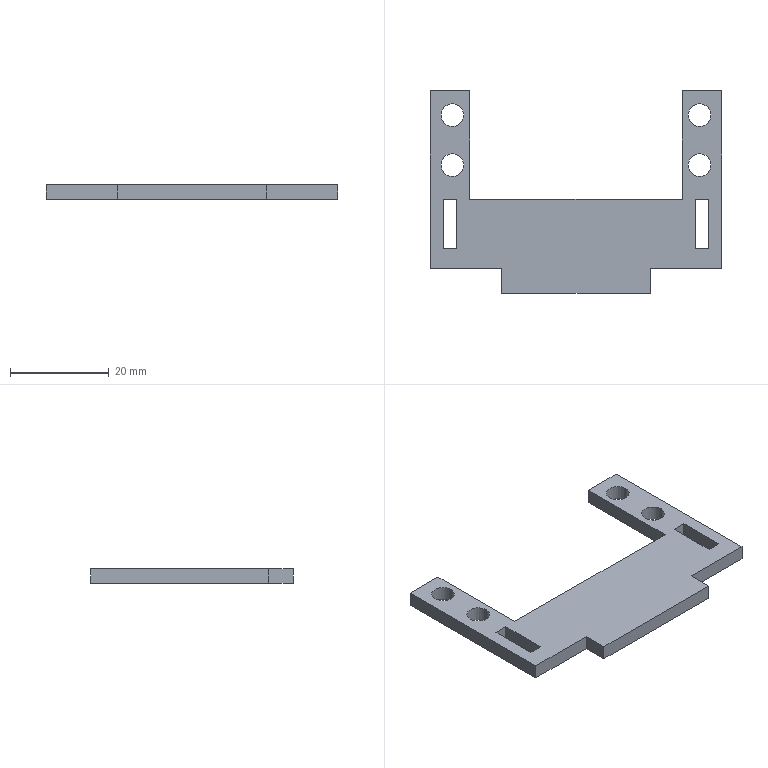Part | SolidWorks | features ICE 2, Extrusion 1 | 1 solid | 30 faces | box 59 x 41 x 3 mm | volume 3617 mm3 | plane 22 | cylinder 8 | commonest cylinder face diameters 4.6 x8
STEP:
#1=CARTESIAN_POINT('',(52.2,-15.05,3.));
#2=VERTEX_POINT('',#1);
#3=CARTESIAN_POINT('',(56.8,-15.05,3.));
#4=VERTEX_POINT('',#3);
#5=CARTESIAN_POINT('',(54.5,-15.05,3.));
#6=DIRECTION('',(0.,0.,1.));
#7=DIRECTION('',(1.,0.,0.));
#8=AXIS2_PLACEMENT_3D('',#5,#6,#7);
#9=CIRCLE('',#8,2.3);
#10=EDGE_CURVE('',#2,#4,#9,.T.);
#11=ORIENTED_EDGE('',*,*,#10,.T.);
#12=CARTESIAN_POINT('',(56.8,-15.05,0.));
#13=VERTEX_POINT('',#12);
#14=CARTESIAN_POINT('',(56.8,-15.05,3.));
#15=DIRECTION('',(0.,0.,-1.));
#16=VECTOR('',#15,1000.);
#17=LINE('',#14,#16);
#18=EDGE_CURVE('',#4,#13,#17,.T.);
#19=ORIENTED_EDGE('',*,*,#18,.T.);
#20=CARTESIAN_POINT('',(52.2,-15.05,0.));
#21=VERTEX_POINT('',#20);
#22=CARTESIAN_POINT('',(54.5,-15.05,0.));
#23=DIRECTION('',(0.,0.,1.));
#24=DIRECTION('',(1.,0.,0.));
#25=AXIS2_PLACEMENT_3D('',#22,#23,#24);
#26=CIRCLE('',#25,2.3);
#27=EDGE_CURVE('',#21,#13,#26,.T.);
#28=ORIENTED_EDGE('',*,*,#27,.F.);
#29=CARTESIAN_POINT('',(52.2,-15.05,3.));
#30=DIRECTION('',(0.,0.,-1.));
#31=VECTOR('',#30,1000.);
#32=LINE('',#29,#31);
#33=EDGE_CURVE('',#2,#21,#32,.T.);
#34=ORIENTED_EDGE('',*,*,#33,.F.);
#35=EDGE_LOOP('',(#11,#19,#28,#34));
#36=FACE_OUTER_BOUND('',#35,.T.);
#37=CARTESIAN_POINT('',(54.5,-15.05,3.));
#38=DIRECTION('',(0.,0.,-1.));
#39=DIRECTION('',(-1.,0.,0.));
#40=AXIS2_PLACEMENT_3D('',#37,#38,#39);
#41=CYLINDRICAL_SURFACE('',#40,2.3);
#42=ADVANCED_FACE('',(#36),#41,.F.);
#43=CARTESIAN_POINT('',(52.2,-4.95,3.));
#44=VERTEX_POINT('',#43);
#45=CARTESIAN_POINT('',(56.8,-4.95,3.));
#46=VERTEX_POINT('',#45);
#47=CARTESIAN_POINT('',(54.5,-4.95,3.));
#48=DIRECTION('',(0.,0.,1.));
#49=DIRECTION('',(1.,0.,0.));
#50=AXIS2_PLACEMENT_3D('',#47,#48,#49);
#51=CIRCLE('',#50,2.3);
#52=EDGE_CURVE('',#44,#46,#51,.T.);
#53=ORIENTED_EDGE('',*,*,#52,.T.);
#54=CARTESIAN_POINT('',(56.8,-4.95,0.));
#55=VERTEX_POINT('',#54);
#56=CARTESIAN_POINT('',(56.8,-4.95,3.));
#57=DIRECTION('',(0.,0.,-1.));
#58=VECTOR('',#57,1000.);
#59=LINE('',#56,#58);
#60=EDGE_CURVE('',#46,#55,#59,.T.);
#61=ORIENTED_EDGE('',*,*,#60,.T.);
#62=CARTESIAN_POINT('',(52.2,-4.95,0.));
#63=VERTEX_POINT('',#62);
#64=CARTESIAN_POINT('',(54.5,-4.95,0.));
#65=DIRECTION('',(0.,0.,1.));
#66=DIRECTION('',(1.,0.,0.));
#67=AXIS2_PLACEMENT_3D('',#64,#65,#66);
#68=CIRCLE('',#67,2.3);
#69=EDGE_CURVE('',#63,#55,#68,.T.);
#70=ORIENTED_EDGE('',*,*,#69,.F.);
#71=CARTESIAN_POINT('',(52.2,-4.95,3.));
#72=DIRECTION('',(0.,0.,-1.));
#73=VECTOR('',#72,1000.);
#74=LINE('',#71,#73);
#75=EDGE_CURVE('',#44,#63,#74,.T.);
#76=ORIENTED_EDGE('',*,*,#75,.F.);
#77=EDGE_LOOP('',(#53,#61,#70,#76));
#78=FACE_OUTER_BOUND('',#77,.T.);
#79=CARTESIAN_POINT('',(54.5,-4.95,3.));
#80=DIRECTION('',(0.,0.,-1.));
#81=DIRECTION('',(-1.,0.,0.));
#82=AXIS2_PLACEMENT_3D('',#79,#80,#81);
#83=CYLINDRICAL_SURFACE('',#82,2.3);
#84=ADVANCED_FACE('',(#78),#83,.F.);
#85=CARTESIAN_POINT('',(2.2,-4.95,3.));
#86=VERTEX_POINT('',#85);
#87=CARTESIAN_POINT('',(6.8,-4.95,3.));
#88=VERTEX_POINT('',#87);
#89=CARTESIAN_POINT('',(4.5,-4.95,3.));
#90=DIRECTION('',(0.,0.,1.));
#91=DIRECTION('',(1.,0.,0.));
#92=AXIS2_PLACEMENT_3D('',#89,#90,#91);
#93=CIRCLE('',#92,2.3);
#94=EDGE_CURVE('',#86,#88,#93,.T.);
#95=ORIENTED_EDGE('',*,*,#94,.T.);
#96=CARTESIAN_POINT('',(6.8,-4.95,0.));
#97=VERTEX_POINT('',#96);
#98=CARTESIAN_POINT('',(6.8,-4.95,3.));
#99=DIRECTION('',(0.,0.,-1.));
#100=VECTOR('',#99,1000.);
#101=LINE('',#98,#100);
#102=EDGE_CURVE('',#88,#97,#101,.T.);
#103=ORIENTED_EDGE('',*,*,#102,.T.);
#104=CARTESIAN_POINT('',(2.2,-4.95,0.));
#105=VERTEX_POINT('',#104);
#106=CARTESIAN_POINT('',(4.5,-4.95,0.));
#107=DIRECTION('',(0.,0.,1.));
#108=DIRECTION('',(1.,0.,0.));
#109=AXIS2_PLACEMENT_3D('',#106,#107,#108);
#110=CIRCLE('',#109,2.3);
#111=EDGE_CURVE('',#105,#97,#110,.T.);
#112=ORIENTED_EDGE('',*,*,#111,.F.);
#113=CARTESIAN_POINT('',(2.2,-4.95,3.));
#114=DIRECTION('',(0.,0.,-1.));
#115=VECTOR('',#114,1000.);
#116=LINE('',#113,#115);
#117=EDGE_CURVE('',#86,#105,#116,.T.);
#118=ORIENTED_EDGE('',*,*,#117,.F.);
#119=EDGE_LOOP('',(#95,#103,#112,#118));
#120=FACE_OUTER_BOUND('',#119,.T.);
#121=CARTESIAN_POINT('',(4.5,-4.95,3.));
#122=DIRECTION('',(0.,0.,-1.));
#123=DIRECTION('',(-1.,0.,0.));
#124=AXIS2_PLACEMENT_3D('',#121,#122,#123);
#125=CYLINDRICAL_SURFACE('',#124,2.3);
#126=ADVANCED_FACE('',(#120),#125,.F.);
#127=CARTESIAN_POINT('',(2.2,-15.05,3.));
#128=VERTEX_POINT('',#127);
#129=CARTESIAN_POINT('',(6.8,-15.05,3.));
#130=VERTEX_POINT('',#129);
#131=CARTESIAN_POINT('',(4.5,-15.05,3.));
#132=DIRECTION('',(0.,0.,1.));
#133=DIRECTION('',(1.,0.,0.));
#134=AXIS2_PLACEMENT_3D('',#131,#132,#133);
#135=CIRCLE('',#134,2.3);
#136=EDGE_CURVE('',#128,#130,#135,.T.);
#137=ORIENTED_EDGE('',*,*,#136,.T.);
#138=CARTESIAN_POINT('',(6.8,-15.05,0.));
#139=VERTEX_POINT('',#138);
#140=CARTESIAN_POINT('',(6.8,-15.05,3.));
#141=DIRECTION('',(0.,0.,-1.));
#142=VECTOR('',#141,1000.);
#143=LINE('',#140,#142);
#144=EDGE_CURVE('',#130,#139,#143,.T.);
#145=ORIENTED_EDGE('',*,*,#144,.T.);
#146=CARTESIAN_POINT('',(2.2,-15.05,0.));
#147=VERTEX_POINT('',#146);
#148=CARTESIAN_POINT('',(4.5,-15.05,0.));
#149=DIRECTION('',(0.,0.,1.));
#150=DIRECTION('',(1.,0.,0.));
#151=AXIS2_PLACEMENT_3D('',#148,#149,#150);
#152=CIRCLE('',#151,2.3);
#153=EDGE_CURVE('',#147,#139,#152,.T.);
#154=ORIENTED_EDGE('',*,*,#153,.F.);
#155=CARTESIAN_POINT('',(2.2,-15.05,3.));
#156=DIRECTION('',(0.,0.,-1.));
#157=VECTOR('',#156,1000.);
#158=LINE('',#155,#157);
#159=EDGE_CURVE('',#128,#147,#158,.T.);
#160=ORIENTED_EDGE('',*,*,#159,.F.);
#161=EDGE_LOOP('',(#137,#145,#154,#160));
#162=FACE_OUTER_BOUND('',#161,.T.);
#163=CARTESIAN_POINT('',(4.5,-15.05,3.));
#164=DIRECTION('',(0.,0.,-1.));
#165=DIRECTION('',(-1.,0.,0.));
#166=AXIS2_PLACEMENT_3D('',#163,#164,#165);
#167=CYLINDRICAL_SURFACE('',#166,2.3);
#168=ADVANCED_FACE('',(#162),#167,.F.);
#169=CARTESIAN_POINT('',(14.5,-36.,3.));
#170=VERTEX_POINT('',#169);
#171=CARTESIAN_POINT('',(14.5,-36.,0.));
#172=VERTEX_POINT('',#171);
#173=CARTESIAN_POINT('',(14.5,-36.,3.));
#174=DIRECTION('',(0.,0.,-1.));
#175=VECTOR('',#174,1000.);
#176=LINE('',#173,#175);
#177=EDGE_CURVE('',#170,#172,#176,.T.);
#178=ORIENTED_EDGE('',*,*,#177,.F.);
#179=CARTESIAN_POINT('',(0.,-36.,3.));
#180=VERTEX_POINT('',#179);
#181=CARTESIAN_POINT('',(0.,-36.,3.));
#182=DIRECTION('',(1.,0.,0.));
#183=VECTOR('',#182,1000.);
#184=LINE('',#181,#183);
#185=EDGE_CURVE('',#180,#170,#184,.T.);
#186=ORIENTED_EDGE('',*,*,#185,.F.);
#187=CARTESIAN_POINT('',(0.,-36.,0.));
#188=VERTEX_POINT('',#187);
#189=CARTESIAN_POINT('',(0.,-36.,3.));
#190=DIRECTION('',(0.,0.,-1.));
#191=VECTOR('',#190,1000.);
#192=LINE('',#189,#191);
#193=EDGE_CURVE('',#180,#188,#192,.T.);
#194=ORIENTED_EDGE('',*,*,#193,.T.);
#195=CARTESIAN_POINT('',(0.,-36.,0.));
#196=DIRECTION('',(1.,0.,0.));
#197=VECTOR('',#196,1000.);
#198=LINE('',#195,#197);
#199=EDGE_CURVE('',#188,#172,#198,.T.);
#200=ORIENTED_EDGE('',*,*,#199,.T.);
#201=EDGE_LOOP('',(#178,#186,#194,#200));
#202=FACE_OUTER_BOUND('',#201,.T.);
#203=CARTESIAN_POINT('',(0.,-36.,3.));
#204=DIRECTION('',(0.,1.,0.));
#205=DIRECTION('',(0.,0.,1.));
#206=AXIS2_PLACEMENT_3D('',#203,#204,#205);
#207=PLANE('',#206);
#208=ADVANCED_FACE('',(#202),#207,.F.);
#209=CARTESIAN_POINT('',(44.5,-36.,0.));
#210=VERTEX_POINT('',#209);
#211=CARTESIAN_POINT('',(44.5,-36.,3.));
#212=VERTEX_POINT('',#211);
#213=CARTESIAN_POINT('',(44.5,-36.,3.));
#214=DIRECTION('',(0.,0.,1.));
#215=VECTOR('',#214,1000.);
#216=LINE('',#213,#215);
#217=EDGE_CURVE('',#210,#212,#216,.T.);
#218=ORIENTED_EDGE('',*,*,#217,.F.);
#219=CARTESIAN_POINT('',(59.,-36.,0.));
#220=VERTEX_POINT('',#219);
#221=CARTESIAN_POINT('',(0.,-36.,0.));
#222=DIRECTION('',(1.,0.,0.));
#223=VECTOR('',#222,1000.);
#224=LINE('',#221,#223);
#225=EDGE_CURVE('',#210,#220,#224,.T.);
#226=ORIENTED_EDGE('',*,*,#225,.T.);
#227=CARTESIAN_POINT('',(59.,-36.,3.));
#228=VERTEX_POINT('',#227);
#229=CARTESIAN_POINT('',(59.,-36.,3.));
#230=DIRECTION('',(0.,0.,-1.));
#231=VECTOR('',#230,1000.);
#232=LINE('',#229,#231);
#233=EDGE_CURVE('',#228,#220,#232,.T.);
#234=ORIENTED_EDGE('',*,*,#233,.F.);
#235=CARTESIAN_POINT('',(0.,-36.,3.));
#236=DIRECTION('',(1.,0.,0.));
#237=VECTOR('',#236,1000.);
#238=LINE('',#235,#237);
#239=EDGE_CURVE('',#212,#228,#238,.T.);
#240=ORIENTED_EDGE('',*,*,#239,.F.);
#241=EDGE_LOOP('',(#218,#226,#234,#240));
#242=FACE_OUTER_BOUND('',#241,.T.);
#243=CARTESIAN_POINT('',(0.,-36.,3.));
#244=DIRECTION('',(0.,1.,0.));
#245=DIRECTION('',(0.,0.,1.));
#246=AXIS2_PLACEMENT_3D('',#243,#244,#245);
#247=PLANE('',#246);
#248=ADVANCED_FACE('',(#242),#247,.F.);
#249=CARTESIAN_POINT('',(51.,0.,0.));
#250=VERTEX_POINT('',#249);
#251=CARTESIAN_POINT('',(59.,0.,0.));
#252=VERTEX_POINT('',#251);
#253=CARTESIAN_POINT('',(0.,0.,0.));
#254=DIRECTION('',(1.,0.,0.));
#255=VECTOR('',#254,1000.);
#256=LINE('',#253,#255);
#257=EDGE_CURVE('',#250,#252,#256,.T.);
#258=ORIENTED_EDGE('',*,*,#257,.F.);
#259=CARTESIAN_POINT('',(51.,0.,3.));
#260=VERTEX_POINT('',#259);
#261=CARTESIAN_POINT('',(51.,0.,3.));
#262=DIRECTION('',(0.,0.,-1.));
#263=VECTOR('',#262,1000.);
#264=LINE('',#261,#263);
#265=EDGE_CURVE('',#260,#250,#264,.T.);
#266=ORIENTED_EDGE('',*,*,#265,.F.);
#267=CARTESIAN_POINT('',(59.,0.,3.));
#268=VERTEX_POINT('',#267);
#269=CARTESIAN_POINT('',(0.,0.,3.));
#270=DIRECTION('',(1.,0.,0.));
#271=VECTOR('',#270,1000.);
#272=LINE('',#269,#271);
#273=EDGE_CURVE('',#260,#268,#272,.T.);
#274=ORIENTED_EDGE('',*,*,#273,.T.);
#275=CARTESIAN_POINT('',(59.,0.,3.));
#276=DIRECTION('',(0.,0.,-1.));
#277=VECTOR('',#276,1000.);
#278=LINE('',#275,#277);
#279=EDGE_CURVE('',#268,#252,#278,.T.);
#280=ORIENTED_EDGE('',*,*,#279,.T.);
#281=EDGE_LOOP('',(#258,#266,#274,#280));
#282=FACE_OUTER_BOUND('',#281,.T.);
#283=CARTESIAN_POINT('',(0.,0.,3.));
#284=DIRECTION('',(0.,1.,0.));
#285=DIRECTION('',(-1.,0.,0.));
#286=AXIS2_PLACEMENT_3D('',#283,#284,#285);
#287=PLANE('',#286);
#288=ADVANCED_FACE('',(#282),#287,.T.);
#289=CARTESIAN_POINT('',(51.,-22.,0.));
#290=VERTEX_POINT('',#289);
#291=CARTESIAN_POINT('',(51.,0.,0.));
#292=DIRECTION('',(0.,1.,0.));
#293=VECTOR('',#292,1000.);
#294=LINE('',#291,#293);
#295=EDGE_CURVE('',#290,#250,#294,.T.);
#296=ORIENTED_EDGE('',*,*,#295,.F.);
#297=CARTESIAN_POINT('',(51.,-22.,3.));
#298=VERTEX_POINT('',#297);
#299=CARTESIAN_POINT('',(51.,-22.,3.));
#300=DIRECTION('',(0.,0.,-1.));
#301=VECTOR('',#300,1000.);
#302=LINE('',#299,#301);
#303=EDGE_CURVE('',#298,#290,#302,.T.);
#304=ORIENTED_EDGE('',*,*,#303,.F.);
#305=CARTESIAN_POINT('',(51.,0.,3.));
#306=DIRECTION('',(0.,1.,0.));
#307=VECTOR('',#306,1000.);
#308=LINE('',#305,#307);
#309=EDGE_CURVE('',#298,#260,#308,.T.);
#310=ORIENTED_EDGE('',*,*,#309,.T.);
#311=ORIENTED_EDGE('',*,*,#265,.T.);
#312=EDGE_LOOP('',(#296,#304,#310,#311));
#313=FACE_OUTER_BOUND('',#312,.T.);
#314=CARTESIAN_POINT('',(51.,0.,3.));
#315=DIRECTION('',(-1.,0.,0.));
#316=DIRECTION('',(0.,0.,1.));
#317=AXIS2_PLACEMENT_3D('',#314,#315,#316);
#318=PLANE('',#317);
#319=ADVANCED_FACE('',(#313),#318,.T.);
#320=CARTESIAN_POINT('',(8.,-22.,0.));
#321=VERTEX_POINT('',#320);
#322=CARTESIAN_POINT('',(0.,-22.,0.));
#323=DIRECTION('',(1.,0.,0.));
#324=VECTOR('',#323,1000.);
#325=LINE('',#322,#324);
#326=EDGE_CURVE('',#321,#290,#325,.T.);
#327=ORIENTED_EDGE('',*,*,#326,.F.);
#328=CARTESIAN_POINT('',(8.,-22.,3.));
#329=VERTEX_POINT('',#328);
#330=CARTESIAN_POINT('',(8.,-22.,3.));
#331=DIRECTION('',(0.,0.,-1.));
#332=VECTOR('',#331,1000.);
#333=LINE('',#330,#332);
#334=EDGE_CURVE('',#329,#321,#333,.T.);
#335=ORIENTED_EDGE('',*,*,#334,.F.);
#336=CARTESIAN_POINT('',(0.,-22.,3.));
#337=DIRECTION('',(1.,0.,0.));
#338=VECTOR('',#337,1000.);
#339=LINE('',#336,#338);
#340=EDGE_CURVE('',#329,#298,#339,.T.);
#341=ORIENTED_EDGE('',*,*,#340,.T.);
#342=ORIENTED_EDGE('',*,*,#303,.T.);
#343=EDGE_LOOP('',(#327,#335,#341,#342));
#344=FACE_OUTER_BOUND('',#343,.T.);
#345=CARTESIAN_POINT('',(0.,-22.,3.));
#346=DIRECTION('',(0.,1.,0.));
#347=DIRECTION('',(0.,0.,1.));
#348=AXIS2_PLACEMENT_3D('',#345,#346,#347);
#349=PLANE('',#348);
#350=ADVANCED_FACE('',(#344),#349,.T.);
#351=CARTESIAN_POINT('',(8.,0.,0.));
#352=VERTEX_POINT('',#351);
#353=CARTESIAN_POINT('',(8.,0.,0.));
#354=DIRECTION('',(0.,-1.,0.));
#355=VECTOR('',#354,1000.);
#356=LINE('',#353,#355);
#357=EDGE_CURVE('',#352,#321,#356,.T.);
#358=ORIENTED_EDGE('',*,*,#357,.F.);
#359=CARTESIAN_POINT('',(8.,0.,3.));
#360=VERTEX_POINT('',#359);
#361=CARTESIAN_POINT('',(8.,0.,3.));
#362=DIRECTION('',(0.,0.,-1.));
#363=VECTOR('',#362,1000.);
#364=LINE('',#361,#363);
#365=EDGE_CURVE('',#360,#352,#364,.T.);
#366=ORIENTED_EDGE('',*,*,#365,.F.);
#367=CARTESIAN_POINT('',(8.,0.,3.));
#368=DIRECTION('',(0.,-1.,0.));
#369=VECTOR('',#368,1000.);
#370=LINE('',#367,#369);
#371=EDGE_CURVE('',#360,#329,#370,.T.);
#372=ORIENTED_EDGE('',*,*,#371,.T.);
#373=ORIENTED_EDGE('',*,*,#334,.T.);
#374=EDGE_LOOP('',(#358,#366,#372,#373));
#375=FACE_OUTER_BOUND('',#374,.T.);
#376=CARTESIAN_POINT('',(8.,0.,3.));
#377=DIRECTION('',(1.,0.,0.));
#378=DIRECTION('',(0.,0.,-1.));
#379=AXIS2_PLACEMENT_3D('',#376,#377,#378);
#380=PLANE('',#379);
#381=ADVANCED_FACE('',(#375),#380,.T.);
#382=CARTESIAN_POINT('',(0.,0.,0.));
#383=VERTEX_POINT('',#382);
#384=CARTESIAN_POINT('',(0.,0.,0.));
#385=DIRECTION('',(1.,0.,0.));
#386=VECTOR('',#385,1000.);
#387=LINE('',#384,#386);
#388=EDGE_CURVE('',#383,#352,#387,.T.);
#389=ORIENTED_EDGE('',*,*,#388,.F.);
#390=CARTESIAN_POINT('',(0.,0.,3.));
#391=VERTEX_POINT('',#390);
#392=CARTESIAN_POINT('',(0.,0.,3.));
#393=DIRECTION('',(0.,0.,-1.));
#394=VECTOR('',#393,1000.);
#395=LINE('',#392,#394);
#396=EDGE_CURVE('',#391,#383,#395,.T.);
#397=ORIENTED_EDGE('',*,*,#396,.F.);
#398=CARTESIAN_POINT('',(0.,0.,3.));
#399=DIRECTION('',(1.,0.,0.));
#400=VECTOR('',#399,1000.);
#401=LINE('',#398,#400);
#402=EDGE_CURVE('',#391,#360,#401,.T.);
#403=ORIENTED_EDGE('',*,*,#402,.T.);
#404=ORIENTED_EDGE('',*,*,#365,.T.);
#405=EDGE_LOOP('',(#389,#397,#403,#404));
#406=FACE_OUTER_BOUND('',#405,.T.);
#407=CARTESIAN_POINT('',(0.,0.,3.));
#408=DIRECTION('',(0.,1.,0.));
#409=DIRECTION('',(0.,0.,1.));
#410=AXIS2_PLACEMENT_3D('',#407,#408,#409);
#411=PLANE('',#410);
#412=ADVANCED_FACE('',(#406),#411,.T.);
#413=CARTESIAN_POINT('',(0.,0.,0.));
#414=DIRECTION('',(0.,-1.,0.));
#415=VECTOR('',#414,1000.);
#416=LINE('',#413,#415);
#417=EDGE_CURVE('',#383,#188,#416,.T.);
#418=ORIENTED_EDGE('',*,*,#417,.T.);
#419=ORIENTED_EDGE('',*,*,#193,.F.);
#420=CARTESIAN_POINT('',(0.,0.,3.));
#421=DIRECTION('',(0.,-1.,0.));
#422=VECTOR('',#421,1000.);
#423=LINE('',#420,#422);
#424=EDGE_CURVE('',#391,#180,#423,.T.);
#425=ORIENTED_EDGE('',*,*,#424,.F.);
#426=ORIENTED_EDGE('',*,*,#396,.T.);
#427=EDGE_LOOP('',(#418,#419,#425,#426));
#428=FACE_OUTER_BOUND('',#427,.T.);
#429=CARTESIAN_POINT('',(0.,0.,3.));
#430=DIRECTION('',(1.,0.,0.));
#431=DIRECTION('',(0.,1.,0.));
#432=AXIS2_PLACEMENT_3D('',#429,#430,#431);
#433=PLANE('',#432);
#434=ADVANCED_FACE('',(#428),#433,.F.);
#435=ORIENTED_EDGE('',*,*,#144,.F.);
#436=CARTESIAN_POINT('',(4.5,-15.05,3.));
#437=DIRECTION('',(0.,0.,1.));
#438=DIRECTION('',(1.,0.,0.));
#439=AXIS2_PLACEMENT_3D('',#436,#437,#438);
#440=CIRCLE('',#439,2.3);
#441=EDGE_CURVE('',#130,#128,#440,.T.);
#442=ORIENTED_EDGE('',*,*,#441,.T.);
#443=ORIENTED_EDGE('',*,*,#159,.T.);
#444=CARTESIAN_POINT('',(4.5,-15.05,0.));
#445=DIRECTION('',(0.,0.,1.));
#446=DIRECTION('',(1.,0.,0.));
#447=AXIS2_PLACEMENT_3D('',#444,#445,#446);
#448=CIRCLE('',#447,2.3);
#449=EDGE_CURVE('',#139,#147,#448,.T.);
#450=ORIENTED_EDGE('',*,*,#449,.F.);
#451=EDGE_LOOP('',(#435,#442,#443,#450));
#452=FACE_OUTER_BOUND('',#451,.T.);
#453=CARTESIAN_POINT('',(4.5,-15.05,3.));
#454=DIRECTION('',(0.,0.,-1.));
#455=DIRECTION('',(-1.,0.,0.));
#456=AXIS2_PLACEMENT_3D('',#453,#454,#455);
#457=CYLINDRICAL_SURFACE('',#456,2.3);
#458=ADVANCED_FACE('',(#452),#457,.F.);
#459=ORIENTED_EDGE('',*,*,#102,.F.);
#460=CARTESIAN_POINT('',(4.5,-4.95,3.));
#461=DIRECTION('',(0.,0.,1.));
#462=DIRECTION('',(1.,0.,0.));
#463=AXIS2_PLACEMENT_3D('',#460,#461,#462);
#464=CIRCLE('',#463,2.3);
#465=EDGE_CURVE('',#88,#86,#464,.T.);
#466=ORIENTED_EDGE('',*,*,#465,.T.);
#467=ORIENTED_EDGE('',*,*,#117,.T.);
#468=CARTESIAN_POINT('',(4.5,-4.95,0.));
#469=DIRECTION('',(0.,0.,1.));
#470=DIRECTION('',(1.,0.,0.));
#471=AXIS2_PLACEMENT_3D('',#468,#469,#470);
#472=CIRCLE('',#471,2.3);
#473=EDGE_CURVE('',#97,#105,#472,.T.);
#474=ORIENTED_EDGE('',*,*,#473,.F.);
#475=EDGE_LOOP('',(#459,#466,#467,#474));
#476=FACE_OUTER_BOUND('',#475,.T.);
#477=CARTESIAN_POINT('',(4.5,-4.95,3.));
#478=DIRECTION('',(0.,0.,-1.));
#479=DIRECTION('',(-1.,0.,0.));
#480=AXIS2_PLACEMENT_3D('',#477,#478,#479);
#481=CYLINDRICAL_SURFACE('',#480,2.3);
#482=ADVANCED_FACE('',(#476),#481,.F.);
#483=ORIENTED_EDGE('',*,*,#60,.F.);
#484=CARTESIAN_POINT('',(54.5,-4.95,3.));
#485=DIRECTION('',(0.,0.,1.));
#486=DIRECTION('',(1.,0.,0.));
#487=AXIS2_PLACEMENT_3D('',#484,#485,#486);
#488=CIRCLE('',#487,2.3);
#489=EDGE_CURVE('',#46,#44,#488,.T.);
#490=ORIENTED_EDGE('',*,*,#489,.T.);
#491=ORIENTED_EDGE('',*,*,#75,.T.);
#492=CARTESIAN_POINT('',(54.5,-4.95,0.));
#493=DIRECTION('',(0.,0.,1.));
#494=DIRECTION('',(1.,0.,0.));
#495=AXIS2_PLACEMENT_3D('',#492,#493,#494);
#496=CIRCLE('',#495,2.3);
#497=EDGE_CURVE('',#55,#63,#496,.T.);
#498=ORIENTED_EDGE('',*,*,#497,.F.);
#499=EDGE_LOOP('',(#483,#490,#491,#498));
#500=FACE_OUTER_BOUND('',#499,.T.);
#501=CARTESIAN_POINT('',(54.5,-4.95,3.));
#502=DIRECTION('',(0.,0.,-1.));
#503=DIRECTION('',(-1.,0.,0.));
#504=AXIS2_PLACEMENT_3D('',#501,#502,#503);
#505=CYLINDRICAL_SURFACE('',#504,2.3);
#506=ADVANCED_FACE('',(#500),#505,.F.);
#507=ORIENTED_EDGE('',*,*,#18,.F.);
#508=CARTESIAN_POINT('',(54.5,-15.05,3.));
#509=DIRECTION('',(0.,0.,1.));
#510=DIRECTION('',(1.,0.,0.));
#511=AXIS2_PLACEMENT_3D('',#508,#509,#510);
#512=CIRCLE('',#511,2.3);
#513=EDGE_CURVE('',#4,#2,#512,.T.);
#514=ORIENTED_EDGE('',*,*,#513,.T.);
#515=ORIENTED_EDGE('',*,*,#33,.T.);
#516=CARTESIAN_POINT('',(54.5,-15.05,0.));
#517=DIRECTION('',(0.,0.,1.));
#518=DIRECTION('',(1.,0.,0.));
#519=AXIS2_PLACEMENT_3D('',#516,#517,#518);
#520=CIRCLE('',#519,2.3);
#521=EDGE_CURVE('',#13,#21,#520,.T.);
#522=ORIENTED_EDGE('',*,*,#521,.F.);
#523=EDGE_LOOP('',(#507,#514,#515,#522));
#524=FACE_OUTER_BOUND('',#523,.T.);
#525=CARTESIAN_POINT('',(54.5,-15.05,3.));
#526=DIRECTION('',(0.,0.,-1.));
#527=DIRECTION('',(-1.,0.,0.));
#528=AXIS2_PLACEMENT_3D('',#525,#526,#527);
#529=CYLINDRICAL_SURFACE('',#528,2.3);
#530=ADVANCED_FACE('',(#524),#529,.F.);
#531=CARTESIAN_POINT('',(59.,0.,0.));
#532=DIRECTION('',(0.,-1.,0.));
#533=VECTOR('',#532,1000.);
#534=LINE('',#531,#533);
#535=EDGE_CURVE('',#252,#220,#534,.T.);
#536=ORIENTED_EDGE('',*,*,#535,.F.);
#537=ORIENTED_EDGE('',*,*,#279,.F.);
#538=CARTESIAN_POINT('',(59.,0.,3.));
#539=DIRECTION('',(0.,-1.,0.));
#540=VECTOR('',#539,1000.);
#541=LINE('',#538,#540);
#542=EDGE_CURVE('',#268,#228,#541,.T.);
#543=ORIENTED_EDGE('',*,*,#542,.T.);
#544=ORIENTED_EDGE('',*,*,#233,.T.);
#545=EDGE_LOOP('',(#536,#537,#543,#544));
#546=FACE_OUTER_BOUND('',#545,.T.);
#547=CARTESIAN_POINT('',(59.,0.,3.));
#548=DIRECTION('',(1.,0.,0.));
#549=DIRECTION('',(0.,1.,0.));
#550=AXIS2_PLACEMENT_3D('',#547,#548,#549);
#551=PLANE('',#550);
#552=ADVANCED_FACE('',(#546),#551,.T.);
#553=CARTESIAN_POINT('',(53.6,-22.,3.));
#554=VERTEX_POINT('',#553);
#555=CARTESIAN_POINT('',(53.6,-32.,3.));
#556=VERTEX_POINT('',#555);
#557=CARTESIAN_POINT('',(53.6,-22.,3.));
#558=DIRECTION('',(0.,-1.,0.));
#559=VECTOR('',#558,1000.);
#560=LINE('',#557,#559);
#561=EDGE_CURVE('',#554,#556,#560,.T.);
#562=ORIENTED_EDGE('',*,*,#561,.F.);
#563=CARTESIAN_POINT('',(56.4,-22.,3.));
#564=VERTEX_POINT('',#563);
#565=CARTESIAN_POINT('',(53.6,-22.,3.));
#566=DIRECTION('',(-1.,0.,0.));
#567=VECTOR('',#566,1000.);
#568=LINE('',#565,#567);
#569=EDGE_CURVE('',#564,#554,#568,.T.);
#570=ORIENTED_EDGE('',*,*,#569,.F.);
#571=CARTESIAN_POINT('',(56.4,-32.,3.));
#572=VERTEX_POINT('',#571);
#573=CARTESIAN_POINT('',(56.4,-22.,3.));
#574=DIRECTION('',(0.,1.,0.));
#575=VECTOR('',#574,1000.);
#576=LINE('',#573,#575);
#577=EDGE_CURVE('',#572,#564,#576,.T.);
#578=ORIENTED_EDGE('',*,*,#577,.F.);
#579=CARTESIAN_POINT('',(53.6,-32.,3.));
#580=DIRECTION('',(1.,0.,0.));
#581=VECTOR('',#580,1000.);
#582=LINE('',#579,#581);
#583=EDGE_CURVE('',#556,#572,#582,.T.);
#584=ORIENTED_EDGE('',*,*,#583,.F.);
#585=EDGE_LOOP('',(#562,#570,#578,#584));
#586=FACE_BOUND('',#585,.T.);
#587=CARTESIAN_POINT('',(2.6,-22.,3.));
#588=VERTEX_POINT('',#587);
#589=CARTESIAN_POINT('',(2.6,-32.,3.));
#590=VERTEX_POINT('',#589);
#591=CARTESIAN_POINT('',(2.6,-22.,3.));
#592=DIRECTION('',(0.,-1.,0.));
#593=VECTOR('',#592,1000.);
#594=LINE('',#591,#593);
#595=EDGE_CURVE('',#588,#590,#594,.T.);
#596=ORIENTED_EDGE('',*,*,#595,.F.);
#597=CARTESIAN_POINT('',(5.4,-22.,3.));
#598=VERTEX_POINT('',#597);
#599=CARTESIAN_POINT('',(2.6,-22.,3.));
#600=DIRECTION('',(-1.,0.,0.));
#601=VECTOR('',#600,1000.);
#602=LINE('',#599,#601);
#603=EDGE_CURVE('',#598,#588,#602,.T.);
#604=ORIENTED_EDGE('',*,*,#603,.F.);
#605=CARTESIAN_POINT('',(5.4,-32.,3.));
#606=VERTEX_POINT('',#605);
#607=CARTESIAN_POINT('',(5.4,-22.,3.));
#608=DIRECTION('',(0.,1.,0.));
#609=VECTOR('',#608,1000.);
#610=LINE('',#607,#609);
#611=EDGE_CURVE('',#606,#598,#610,.T.);
#612=ORIENTED_EDGE('',*,*,#611,.F.);
#613=CARTESIAN_POINT('',(2.6,-32.,3.));
#614=DIRECTION('',(1.,0.,0.));
#615=VECTOR('',#614,1000.);
#616=LINE('',#613,#615);
#617=EDGE_CURVE('',#590,#606,#616,.T.);
#618=ORIENTED_EDGE('',*,*,#617,.F.);
#619=EDGE_LOOP('',(#596,#604,#612,#618));
#620=FACE_BOUND('',#619,.T.);
#621=ORIENTED_EDGE('',*,*,#10,.F.);
#622=ORIENTED_EDGE('',*,*,#513,.F.);
#623=EDGE_LOOP('',(#621,#622));
#624=FACE_BOUND('',#623,.T.);
#625=ORIENTED_EDGE('',*,*,#52,.F.);
#626=ORIENTED_EDGE('',*,*,#489,.F.);
#627=EDGE_LOOP('',(#625,#626));
#628=FACE_BOUND('',#627,.T.);
#629=ORIENTED_EDGE('',*,*,#94,.F.);
#630=ORIENTED_EDGE('',*,*,#465,.F.);
#631=EDGE_LOOP('',(#629,#630));
#632=FACE_BOUND('',#631,.T.);
#633=ORIENTED_EDGE('',*,*,#136,.F.);
#634=ORIENTED_EDGE('',*,*,#441,.F.);
#635=EDGE_LOOP('',(#633,#634));
#636=FACE_BOUND('',#635,.T.);
#637=ORIENTED_EDGE('',*,*,#273,.F.);
#638=ORIENTED_EDGE('',*,*,#309,.F.);
#639=ORIENTED_EDGE('',*,*,#340,.F.);
#640=ORIENTED_EDGE('',*,*,#371,.F.);
#641=ORIENTED_EDGE('',*,*,#402,.F.);
#642=ORIENTED_EDGE('',*,*,#424,.T.);
#643=ORIENTED_EDGE('',*,*,#185,.T.);
#644=CARTESIAN_POINT('',(14.5,-41.,3.));
#645=VERTEX_POINT('',#644);
#646=CARTESIAN_POINT('',(14.5,-41.,3.));
#647=DIRECTION('',(0.,1.,0.));
#648=VECTOR('',#647,1000.);
#649=LINE('',#646,#648);
#650=EDGE_CURVE('',#645,#170,#649,.T.);
#651=ORIENTED_EDGE('',*,*,#650,.F.);
#652=CARTESIAN_POINT('',(44.5,-41.,3.));
#653=VERTEX_POINT('',#652);
#654=CARTESIAN_POINT('',(14.5,-41.,3.));
#655=DIRECTION('',(-1.,0.,0.));
#656=VECTOR('',#655,1000.);
#657=LINE('',#654,#656);
#658=EDGE_CURVE('',#653,#645,#657,.T.);
#659=ORIENTED_EDGE('',*,*,#658,.F.);
#660=CARTESIAN_POINT('',(44.5,-41.,3.));
#661=DIRECTION('',(0.,1.,0.));
#662=VECTOR('',#661,1000.);
#663=LINE('',#660,#662);
#664=EDGE_CURVE('',#653,#212,#663,.T.);
#665=ORIENTED_EDGE('',*,*,#664,.T.);
#666=ORIENTED_EDGE('',*,*,#239,.T.);
#667=ORIENTED_EDGE('',*,*,#542,.F.);
#668=EDGE_LOOP('',(#637,#638,#639,#640,#641,#642,#643,#651,#659,#665,#666,#667));
#669=FACE_OUTER_BOUND('',#668,.T.);
#670=CARTESIAN_POINT('',(0.,0.,3.));
#671=DIRECTION('',(0.,0.,1.));
#672=DIRECTION('',(1.,0.,0.));
#673=AXIS2_PLACEMENT_3D('',#670,#671,#672);
#674=PLANE('',#673);
#675=ADVANCED_FACE('',(#586,#620,#624,#628,#632,#636,#669),#674,.T.);
#676=CARTESIAN_POINT('',(56.4,-22.,0.));
#677=VERTEX_POINT('',#676);
#678=CARTESIAN_POINT('',(53.6,-22.,0.));
#679=VERTEX_POINT('',#678);
#680=CARTESIAN_POINT('',(0.,-22.,0.));
#681=DIRECTION('',(-1.,0.,0.));
#682=VECTOR('',#681,1000.);
#683=LINE('',#680,#682);
#684=EDGE_CURVE('',#677,#679,#683,.T.);
#685=ORIENTED_EDGE('',*,*,#684,.T.);
#686=CARTESIAN_POINT('',(53.6,-32.,0.));
#687=VERTEX_POINT('',#686);
#688=CARTESIAN_POINT('',(53.6,0.,0.));
#689=DIRECTION('',(0.,-1.,0.));
#690=VECTOR('',#689,1000.);
#691=LINE('',#688,#690);
#692=EDGE_CURVE('',#679,#687,#691,.T.);
#693=ORIENTED_EDGE('',*,*,#692,.T.);
#694=CARTESIAN_POINT('',(56.4,-32.,0.));
#695=VERTEX_POINT('',#694);
#696=CARTESIAN_POINT('',(0.,-32.,0.));
#697=DIRECTION('',(1.,0.,0.));
#698=VECTOR('',#697,1000.);
#699=LINE('',#696,#698);
#700=EDGE_CURVE('',#687,#695,#699,.T.);
#701=ORIENTED_EDGE('',*,*,#700,.T.);
#702=CARTESIAN_POINT('',(56.4,0.,0.));
#703=DIRECTION('',(0.,1.,0.));
#704=VECTOR('',#703,1000.);
#705=LINE('',#702,#704);
#706=EDGE_CURVE('',#695,#677,#705,.T.);
#707=ORIENTED_EDGE('',*,*,#706,.T.);
#708=EDGE_LOOP('',(#685,#693,#701,#707));
#709=FACE_BOUND('',#708,.T.);
#710=CARTESIAN_POINT('',(5.4,-22.,0.));
#711=VERTEX_POINT('',#710);
#712=CARTESIAN_POINT('',(2.6,-22.,0.));
#713=VERTEX_POINT('',#712);
#714=CARTESIAN_POINT('',(0.,-22.,0.));
#715=DIRECTION('',(-1.,0.,0.));
#716=VECTOR('',#715,1000.);
#717=LINE('',#714,#716);
#718=EDGE_CURVE('',#711,#713,#717,.T.);
#719=ORIENTED_EDGE('',*,*,#718,.T.);
#720=CARTESIAN_POINT('',(2.6,-32.,0.));
#721=VERTEX_POINT('',#720);
#722=CARTESIAN_POINT('',(2.6,0.,0.));
#723=DIRECTION('',(0.,-1.,0.));
#724=VECTOR('',#723,1000.);
#725=LINE('',#722,#724);
#726=EDGE_CURVE('',#713,#721,#725,.T.);
#727=ORIENTED_EDGE('',*,*,#726,.T.);
#728=CARTESIAN_POINT('',(5.4,-32.,0.));
#729=VERTEX_POINT('',#728);
#730=CARTESIAN_POINT('',(0.,-32.,0.));
#731=DIRECTION('',(1.,0.,0.));
#732=VECTOR('',#731,1000.);
#733=LINE('',#730,#732);
#734=EDGE_CURVE('',#721,#729,#733,.T.);
#735=ORIENTED_EDGE('',*,*,#734,.T.);
#736=CARTESIAN_POINT('',(5.4,0.,0.));
#737=DIRECTION('',(0.,1.,0.));
#738=VECTOR('',#737,1000.);
#739=LINE('',#736,#738);
#740=EDGE_CURVE('',#729,#711,#739,.T.);
#741=ORIENTED_EDGE('',*,*,#740,.T.);
#742=EDGE_LOOP('',(#719,#727,#735,#741));
#743=FACE_BOUND('',#742,.T.);
#744=ORIENTED_EDGE('',*,*,#27,.T.);
#745=ORIENTED_EDGE('',*,*,#521,.T.);
#746=EDGE_LOOP('',(#744,#745));
#747=FACE_BOUND('',#746,.T.);
#748=ORIENTED_EDGE('',*,*,#69,.T.);
#749=ORIENTED_EDGE('',*,*,#497,.T.);
#750=EDGE_LOOP('',(#748,#749));
#751=FACE_BOUND('',#750,.T.);
#752=ORIENTED_EDGE('',*,*,#111,.T.);
#753=ORIENTED_EDGE('',*,*,#473,.T.);
#754=EDGE_LOOP('',(#752,#753));
#755=FACE_BOUND('',#754,.T.);
#756=ORIENTED_EDGE('',*,*,#153,.T.);
#757=ORIENTED_EDGE('',*,*,#449,.T.);
#758=EDGE_LOOP('',(#756,#757));
#759=FACE_BOUND('',#758,.T.);
#760=ORIENTED_EDGE('',*,*,#257,.T.);
#761=ORIENTED_EDGE('',*,*,#535,.T.);
#762=ORIENTED_EDGE('',*,*,#225,.F.);
#763=CARTESIAN_POINT('',(44.5,-41.,0.));
#764=VERTEX_POINT('',#763);
#765=CARTESIAN_POINT('',(44.5,-41.,0.));
#766=DIRECTION('',(0.,1.,0.));
#767=VECTOR('',#766,1000.);
#768=LINE('',#765,#767);
#769=EDGE_CURVE('',#764,#210,#768,.T.);
#770=ORIENTED_EDGE('',*,*,#769,.F.);
#771=CARTESIAN_POINT('',(14.5,-41.,0.));
#772=VERTEX_POINT('',#771);
#773=CARTESIAN_POINT('',(14.5,-41.,0.));
#774=DIRECTION('',(1.,0.,0.));
#775=VECTOR('',#774,1000.);
#776=LINE('',#773,#775);
#777=EDGE_CURVE('',#772,#764,#776,.T.);
#778=ORIENTED_EDGE('',*,*,#777,.F.);
#779=CARTESIAN_POINT('',(14.5,-41.,0.));
#780=DIRECTION('',(0.,1.,0.));
#781=VECTOR('',#780,1000.);
#782=LINE('',#779,#781);
#783=EDGE_CURVE('',#772,#172,#782,.T.);
#784=ORIENTED_EDGE('',*,*,#783,.T.);
#785=ORIENTED_EDGE('',*,*,#199,.F.);
#786=ORIENTED_EDGE('',*,*,#417,.F.);
#787=ORIENTED_EDGE('',*,*,#388,.T.);
#788=ORIENTED_EDGE('',*,*,#357,.T.);
#789=ORIENTED_EDGE('',*,*,#326,.T.);
#790=ORIENTED_EDGE('',*,*,#295,.T.);
#791=EDGE_LOOP('',(#760,#761,#762,#770,#778,#784,#785,#786,#787,#788,#789,#790));
#792=FACE_OUTER_BOUND('',#791,.T.);
#793=CARTESIAN_POINT('',(0.,0.,0.));
#794=DIRECTION('',(0.,0.,1.));
#795=DIRECTION('',(1.,0.,0.));
#796=AXIS2_PLACEMENT_3D('',#793,#794,#795);
#797=PLANE('',#796);
#798=ADVANCED_FACE('',(#709,#743,#747,#751,#755,#759,#792),#797,.F.);
#799=CARTESIAN_POINT('',(2.6,-22.,-7.));
#800=DIRECTION('',(0.,0.,1.));
#801=VECTOR('',#800,1000.);
#802=LINE('',#799,#801);
#803=EDGE_CURVE('',#713,#588,#802,.T.);
#804=ORIENTED_EDGE('',*,*,#803,.T.);
#805=ORIENTED_EDGE('',*,*,#595,.T.);
#806=CARTESIAN_POINT('',(2.6,-32.,-7.));
#807=DIRECTION('',(0.,0.,1.));
#808=VECTOR('',#807,1000.);
#809=LINE('',#806,#808);
#810=EDGE_CURVE('',#721,#590,#809,.T.);
#811=ORIENTED_EDGE('',*,*,#810,.F.);
#812=ORIENTED_EDGE('',*,*,#726,.F.);
#813=EDGE_LOOP('',(#804,#805,#811,#812));
#814=FACE_OUTER_BOUND('',#813,.T.);
#815=CARTESIAN_POINT('',(2.6,-22.,-7.));
#816=DIRECTION('',(-1.,0.,0.));
#817=DIRECTION('',(0.,-1.,0.));
#818=AXIS2_PLACEMENT_3D('',#815,#816,#817);
#819=PLANE('',#818);
#820=ADVANCED_FACE('',(#814),#819,.F.);
#821=CARTESIAN_POINT('',(5.4,-22.,-7.));
#822=DIRECTION('',(0.,0.,1.));
#823=VECTOR('',#822,1000.);
#824=LINE('',#821,#823);
#825=EDGE_CURVE('',#711,#598,#824,.T.);
#826=ORIENTED_EDGE('',*,*,#825,.T.);
#827=ORIENTED_EDGE('',*,*,#603,.T.);
#828=ORIENTED_EDGE('',*,*,#803,.F.);
#829=ORIENTED_EDGE('',*,*,#718,.F.);
#830=EDGE_LOOP('',(#826,#827,#828,#829));
#831=FACE_OUTER_BOUND('',#830,.T.);
#832=CARTESIAN_POINT('',(2.6,-22.,-7.));
#833=DIRECTION('',(0.,1.,0.));
#834=DIRECTION('',(-1.,0.,0.));
#835=AXIS2_PLACEMENT_3D('',#832,#833,#834);
#836=PLANE('',#835);
#837=ADVANCED_FACE('',(#831),#836,.F.);
#838=CARTESIAN_POINT('',(5.4,-32.,-7.));
#839=DIRECTION('',(0.,0.,1.));
#840=VECTOR('',#839,1000.);
#841=LINE('',#838,#840);
#842=EDGE_CURVE('',#729,#606,#841,.T.);
#843=ORIENTED_EDGE('',*,*,#842,.T.);
#844=ORIENTED_EDGE('',*,*,#611,.T.);
#845=ORIENTED_EDGE('',*,*,#825,.F.);
#846=ORIENTED_EDGE('',*,*,#740,.F.);
#847=EDGE_LOOP('',(#843,#844,#845,#846));
#848=FACE_OUTER_BOUND('',#847,.T.);
#849=CARTESIAN_POINT('',(5.4,-22.,-7.));
#850=DIRECTION('',(1.,0.,0.));
#851=DIRECTION('',(0.,1.,0.));
#852=AXIS2_PLACEMENT_3D('',#849,#850,#851);
#853=PLANE('',#852);
#854=ADVANCED_FACE('',(#848),#853,.F.);
#855=ORIENTED_EDGE('',*,*,#810,.T.);
#856=ORIENTED_EDGE('',*,*,#617,.T.);
#857=ORIENTED_EDGE('',*,*,#842,.F.);
#858=ORIENTED_EDGE('',*,*,#734,.F.);
#859=EDGE_LOOP('',(#855,#856,#857,#858));
#860=FACE_OUTER_BOUND('',#859,.T.);
#861=CARTESIAN_POINT('',(2.6,-32.,-7.));
#862=DIRECTION('',(0.,-1.,0.));
#863=DIRECTION('',(0.,0.,-1.));
#864=AXIS2_PLACEMENT_3D('',#861,#862,#863);
#865=PLANE('',#864);
#866=ADVANCED_FACE('',(#860),#865,.F.);
#867=CARTESIAN_POINT('',(53.6,-22.,-7.));
#868=DIRECTION('',(0.,0.,1.));
#869=VECTOR('',#868,1000.);
#870=LINE('',#867,#869);
#871=EDGE_CURVE('',#679,#554,#870,.T.);
#872=ORIENTED_EDGE('',*,*,#871,.T.);
#873=ORIENTED_EDGE('',*,*,#561,.T.);
#874=CARTESIAN_POINT('',(53.6,-32.,-7.));
#875=DIRECTION('',(0.,0.,1.));
#876=VECTOR('',#875,1000.);
#877=LINE('',#874,#876);
#878=EDGE_CURVE('',#687,#556,#877,.T.);
#879=ORIENTED_EDGE('',*,*,#878,.F.);
#880=ORIENTED_EDGE('',*,*,#692,.F.);
#881=EDGE_LOOP('',(#872,#873,#879,#880));
#882=FACE_OUTER_BOUND('',#881,.T.);
#883=CARTESIAN_POINT('',(53.6,-22.,-7.));
#884=DIRECTION('',(-1.,0.,0.));
#885=DIRECTION('',(0.,-1.,0.));
#886=AXIS2_PLACEMENT_3D('',#883,#884,#885);
#887=PLANE('',#886);
#888=ADVANCED_FACE('',(#882),#887,.F.);
#889=CARTESIAN_POINT('',(56.4,-22.,-7.));
#890=DIRECTION('',(0.,0.,1.));
#891=VECTOR('',#890,1000.);
#892=LINE('',#889,#891);
#893=EDGE_CURVE('',#677,#564,#892,.T.);
#894=ORIENTED_EDGE('',*,*,#893,.T.);
#895=ORIENTED_EDGE('',*,*,#569,.T.);
#896=ORIENTED_EDGE('',*,*,#871,.F.);
#897=ORIENTED_EDGE('',*,*,#684,.F.);
#898=EDGE_LOOP('',(#894,#895,#896,#897));
#899=FACE_OUTER_BOUND('',#898,.T.);
#900=CARTESIAN_POINT('',(53.6,-22.,-7.));
#901=DIRECTION('',(0.,1.,0.));
#902=DIRECTION('',(0.,0.,1.));
#903=AXIS2_PLACEMENT_3D('',#900,#901,#902);
#904=PLANE('',#903);
#905=ADVANCED_FACE('',(#899),#904,.F.);
#906=CARTESIAN_POINT('',(56.4,-32.,-7.));
#907=DIRECTION('',(0.,0.,1.));
#908=VECTOR('',#907,1000.);
#909=LINE('',#906,#908);
#910=EDGE_CURVE('',#695,#572,#909,.T.);
#911=ORIENTED_EDGE('',*,*,#910,.T.);
#912=ORIENTED_EDGE('',*,*,#577,.T.);
#913=ORIENTED_EDGE('',*,*,#893,.F.);
#914=ORIENTED_EDGE('',*,*,#706,.F.);
#915=EDGE_LOOP('',(#911,#912,#913,#914));
#916=FACE_OUTER_BOUND('',#915,.T.);
#917=CARTESIAN_POINT('',(56.4,-22.,-7.));
#918=DIRECTION('',(1.,0.,0.));
#919=DIRECTION('',(0.,0.,-1.));
#920=AXIS2_PLACEMENT_3D('',#917,#918,#919);
#921=PLANE('',#920);
#922=ADVANCED_FACE('',(#916),#921,.F.);
#923=ORIENTED_EDGE('',*,*,#878,.T.);
#924=ORIENTED_EDGE('',*,*,#583,.T.);
#925=ORIENTED_EDGE('',*,*,#910,.F.);
#926=ORIENTED_EDGE('',*,*,#700,.F.);
#927=EDGE_LOOP('',(#923,#924,#925,#926));
#928=FACE_OUTER_BOUND('',#927,.T.);
#929=CARTESIAN_POINT('',(53.6,-32.,-7.));
#930=DIRECTION('',(0.,-1.,0.));
#931=DIRECTION('',(0.,0.,-1.));
#932=AXIS2_PLACEMENT_3D('',#929,#930,#931);
#933=PLANE('',#932);
#934=ADVANCED_FACE('',(#928),#933,.F.);
#935=ORIENTED_EDGE('',*,*,#177,.T.);
#936=ORIENTED_EDGE('',*,*,#783,.F.);
#937=CARTESIAN_POINT('',(14.5,-41.,3.));
#938=DIRECTION('',(0.,0.,-1.));
#939=VECTOR('',#938,1000.);
#940=LINE('',#937,#939);
#941=EDGE_CURVE('',#645,#772,#940,.T.);
#942=ORIENTED_EDGE('',*,*,#941,.F.);
#943=ORIENTED_EDGE('',*,*,#650,.T.);
#944=EDGE_LOOP('',(#935,#936,#942,#943));
#945=FACE_OUTER_BOUND('',#944,.T.);
#946=CARTESIAN_POINT('',(14.5,-41.,3.));
#947=DIRECTION('',(1.,0.,0.));
#948=DIRECTION('',(0.,0.,-1.));
#949=AXIS2_PLACEMENT_3D('',#946,#947,#948);
#950=PLANE('',#949);
#951=ADVANCED_FACE('',(#945),#950,.F.);
#952=ORIENTED_EDGE('',*,*,#217,.T.);
#953=ORIENTED_EDGE('',*,*,#664,.F.);
#954=CARTESIAN_POINT('',(44.5,-41.,3.));
#955=DIRECTION('',(0.,0.,1.));
#956=VECTOR('',#955,1000.);
#957=LINE('',#954,#956);
#958=EDGE_CURVE('',#764,#653,#957,.T.);
#959=ORIENTED_EDGE('',*,*,#958,.F.);
#960=ORIENTED_EDGE('',*,*,#769,.T.);
#961=EDGE_LOOP('',(#952,#953,#959,#960));
#962=FACE_OUTER_BOUND('',#961,.T.);
#963=CARTESIAN_POINT('',(44.5,-41.,3.));
#964=DIRECTION('',(-1.,0.,0.));
#965=DIRECTION('',(0.,0.,1.));
#966=AXIS2_PLACEMENT_3D('',#963,#964,#965);
#967=PLANE('',#966);
#968=ADVANCED_FACE('',(#962),#967,.F.);
#969=ORIENTED_EDGE('',*,*,#941,.T.);
#970=ORIENTED_EDGE('',*,*,#777,.T.);
#971=ORIENTED_EDGE('',*,*,#958,.T.);
#972=ORIENTED_EDGE('',*,*,#658,.T.);
#973=EDGE_LOOP('',(#969,#970,#971,#972));
#974=FACE_OUTER_BOUND('',#973,.T.);
#975=CARTESIAN_POINT('',(0.,-41.,0.));
#976=DIRECTION('',(0.,-1.,0.));
#977=DIRECTION('',(0.,0.,-1.));
#978=AXIS2_PLACEMENT_3D('',#975,#976,#977);
#979=PLANE('',#978);
#980=ADVANCED_FACE('',(#974),#979,.T.);
#981=CLOSED_SHELL('',(#42,#84,#126,#168,#208,#248,#288,#319,#350,#381,#412,#434,#458,#482,#506,#530,#552,#675,#798,#820,#837,#854,#866,#888,#905,#922,#934,#951,#968,#980));
#982=MANIFOLD_SOLID_BREP('',#981);
#983=CARTESIAN_POINT('',(0.,0.,0.));
#984=DIRECTION('',(0.,0.,1.));
#985=DIRECTION('',(1.,0.,0.));
#986=AXIS2_PLACEMENT_3D('',#983,#984,#985);
#987=(LENGTH_UNIT()NAMED_UNIT(*)SI_UNIT(.MILLI.,.METRE.));
#988=UNCERTAINTY_MEASURE_WITH_UNIT(LENGTH_MEASURE(0.00001),#987,'','');
#989=(NAMED_UNIT(*)PLANE_ANGLE_UNIT()SI_UNIT($,.RADIAN.));
#990=(NAMED_UNIT(*)SI_UNIT($,.STERADIAN.)SOLID_ANGLE_UNIT());
#991=(GEOMETRIC_REPRESENTATION_CONTEXT(3)GLOBAL_UNCERTAINTY_ASSIGNED_CONTEXT((#988))GLOBAL_UNIT_ASSIGNED_CONTEXT((#987,#989,#990))REPRESENTATION_CONTEXT('',''));
#992=ADVANCED_BREP_SHAPE_REPRESENTATION('',(#982,#986),#991);